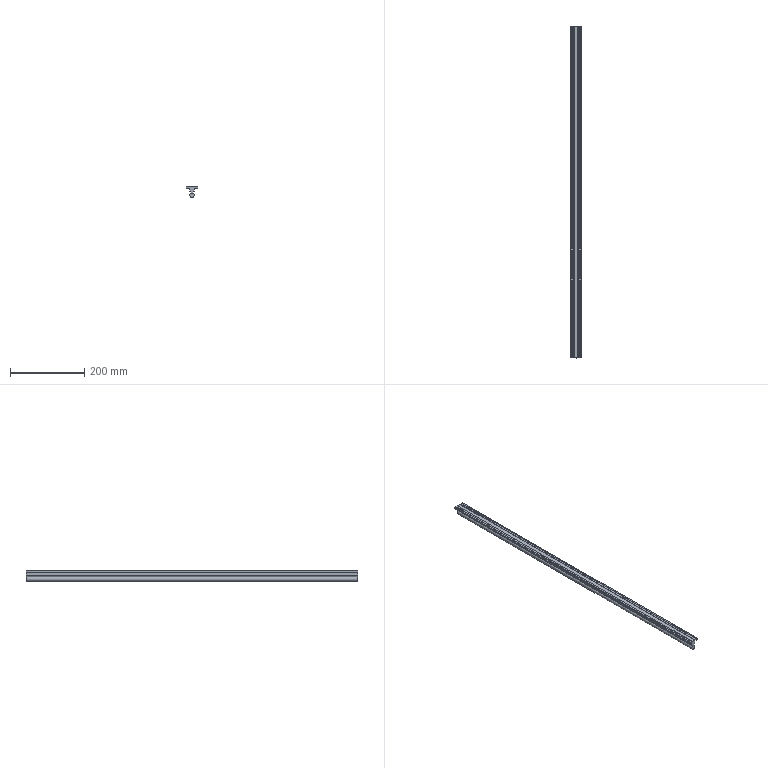Part | SolidWorks | features BaseBody 1 | 1 solid | 127 faces | box 30 x 895 x 28.5 mm | volume 320903 mm3 | plane 93 | cylinder 34 | commonest cylinder face diameters 4.5 x32 12 x2